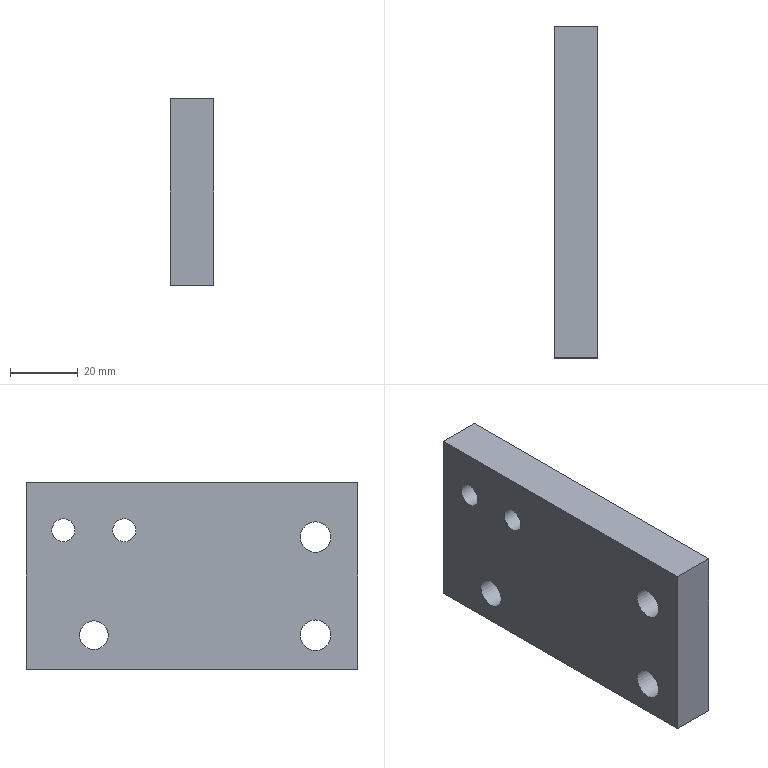Part | NX | features LIN_SOLID_COLOR 2 | 1 solid | 11 faces | box 13 x 98 x 55 mm | volume 66734 mm3 | plane 6 | cylinder 5 | commonest cylinder face diameters 6.8 x2 9 x2 8.5 x1
STEP:
#1=CARTESIAN_POINT('',(938.,-60.,21.25));
#2=VERTEX_POINT('',#1);
#3=CARTESIAN_POINT('',(938.,-60.,17.));
#4=DIRECTION('',(-1.,0.,0.));
#5=DIRECTION('',(0.,0.,1.));
#6=AXIS2_PLACEMENT_3D('',#3,#4,#5);
#7=CIRCLE('',#6,4.25);
#8=EDGE_CURVE('',#2,#2,#7,.T.);
#9=ORIENTED_EDGE('',*,*,#8,.T.);
#10=EDGE_LOOP('',(#9));
#11=FACE_BOUND('',#10,.T.);
#12=CARTESIAN_POINT('',(951.,-60.,12.75));
#13=VERTEX_POINT('',#12);
#14=CARTESIAN_POINT('',(951.,-60.,17.));
#15=DIRECTION('',(1.,0.,0.));
#16=DIRECTION('',(0.,0.,-1.));
#17=AXIS2_PLACEMENT_3D('',#14,#15,#16);
#18=CIRCLE('',#17,4.25);
#19=EDGE_CURVE('',#13,#13,#18,.F.);
#20=ORIENTED_EDGE('',*,*,#19,.F.);
#21=EDGE_LOOP('',(#20));
#22=FACE_BOUND('',#21,.T.);
#23=CARTESIAN_POINT('',(951.,-60.,17.));
#24=DIRECTION('',(-1.,0.,0.));
#25=DIRECTION('',(0.,0.,-1.));
#26=AXIS2_PLACEMENT_3D('',#23,#24,#25);
#27=CYLINDRICAL_SURFACE('',#26,4.25);
#28=ADVANCED_FACE('',(#11,#22),#27,.F.);
#29=CARTESIAN_POINT('',(938.,-69.,51.4));
#30=VERTEX_POINT('',#29);
#31=CARTESIAN_POINT('',(938.,-69.,48.));
#32=DIRECTION('',(-1.,0.,0.));
#33=DIRECTION('',(0.,0.,1.));
#34=AXIS2_PLACEMENT_3D('',#31,#32,#33);
#35=CIRCLE('',#34,3.4);
#36=EDGE_CURVE('',#30,#30,#35,.T.);
#37=ORIENTED_EDGE('',*,*,#36,.T.);
#38=EDGE_LOOP('',(#37));
#39=FACE_BOUND('',#38,.T.);
#40=CARTESIAN_POINT('',(951.,-69.,44.6));
#41=VERTEX_POINT('',#40);
#42=CARTESIAN_POINT('',(951.,-69.,48.));
#43=DIRECTION('',(1.,0.,0.));
#44=DIRECTION('',(0.,0.,-1.));
#45=AXIS2_PLACEMENT_3D('',#42,#43,#44);
#46=CIRCLE('',#45,3.4);
#47=EDGE_CURVE('',#41,#41,#46,.F.);
#48=ORIENTED_EDGE('',*,*,#47,.F.);
#49=EDGE_LOOP('',(#48));
#50=FACE_BOUND('',#49,.T.);
#51=CARTESIAN_POINT('',(951.,-69.,48.));
#52=DIRECTION('',(-1.,0.,0.));
#53=DIRECTION('',(0.,0.,-1.));
#54=AXIS2_PLACEMENT_3D('',#51,#52,#53);
#55=CYLINDRICAL_SURFACE('',#54,3.4);
#56=ADVANCED_FACE('',(#39,#50),#55,.F.);
#57=CARTESIAN_POINT('',(951.,-138.,7.));
#58=VERTEX_POINT('',#57);
#59=CARTESIAN_POINT('',(951.,-138.,62.));
#60=VERTEX_POINT('',#59);
#61=CARTESIAN_POINT('',(951.,-138.,33.449));
#62=DIRECTION('',(0.,0.,-1.));
#63=VECTOR('',#62,1000.);
#64=LINE('',#61,#63);
#65=EDGE_CURVE('',#58,#60,#64,.F.);
#66=ORIENTED_EDGE('',*,*,#65,.T.);
#67=CARTESIAN_POINT('',(938.,-138.,62.));
#68=VERTEX_POINT('',#67);
#69=CARTESIAN_POINT('',(938.5,-138.,62.));
#70=DIRECTION('',(-1.,0.,0.));
#71=VECTOR('',#70,1000.);
#72=LINE('',#69,#71);
#73=EDGE_CURVE('',#60,#68,#72,.T.);
#74=ORIENTED_EDGE('',*,*,#73,.T.);
#75=CARTESIAN_POINT('',(938.,-138.,7.));
#76=VERTEX_POINT('',#75);
#77=CARTESIAN_POINT('',(938.,-138.,33.449));
#78=DIRECTION('',(0.,0.,-1.));
#79=VECTOR('',#78,1000.);
#80=LINE('',#77,#79);
#81=EDGE_CURVE('',#76,#68,#80,.F.);
#82=ORIENTED_EDGE('',*,*,#81,.F.);
#83=CARTESIAN_POINT('',(938.5,-138.,7.));
#84=DIRECTION('',(1.,0.,0.));
#85=VECTOR('',#84,1000.);
#86=LINE('',#83,#85);
#87=EDGE_CURVE('',#76,#58,#86,.T.);
#88=ORIENTED_EDGE('',*,*,#87,.T.);
#89=EDGE_LOOP('',(#66,#74,#82,#88));
#90=FACE_BOUND('',#89,.T.);
#91=CARTESIAN_POINT('',(938.5,-138.,33.449));
#92=DIRECTION('',(0.,-1.,0.));
#93=DIRECTION('',(0.,0.,1.));
#94=AXIS2_PLACEMENT_3D('',#91,#92,#93);
#95=PLANE('',#94);
#96=ADVANCED_FACE('',(#90),#95,.T.);
#97=CARTESIAN_POINT('',(951.,-40.,7.));
#98=VERTEX_POINT('',#97);
#99=CARTESIAN_POINT('',(951.,-175.,7.));
#100=DIRECTION('',(0.,1.,0.));
#101=VECTOR('',#100,1000.);
#102=LINE('',#99,#101);
#103=EDGE_CURVE('',#58,#98,#102,.T.);
#104=ORIENTED_EDGE('',*,*,#103,.F.);
#105=ORIENTED_EDGE('',*,*,#87,.F.);
#106=CARTESIAN_POINT('',(938.,-40.,7.));
#107=VERTEX_POINT('',#106);
#108=CARTESIAN_POINT('',(938.,-175.,7.));
#109=DIRECTION('',(0.,-1.,0.));
#110=VECTOR('',#109,1000.);
#111=LINE('',#108,#110);
#112=EDGE_CURVE('',#107,#76,#111,.T.);
#113=ORIENTED_EDGE('',*,*,#112,.F.);
#114=CARTESIAN_POINT('',(973.,-40.,7.));
#115=DIRECTION('',(-1.,0.,0.));
#116=VECTOR('',#115,1000.);
#117=LINE('',#114,#116);
#118=EDGE_CURVE('',#98,#107,#117,.T.);
#119=ORIENTED_EDGE('',*,*,#118,.F.);
#120=EDGE_LOOP('',(#104,#105,#113,#119));
#121=FACE_BOUND('',#120,.T.);
#122=CARTESIAN_POINT('',(948.5,-25.,7.));
#123=DIRECTION('',(0.,0.,1.));
#124=DIRECTION('',(0.,-1.,0.));
#125=AXIS2_PLACEMENT_3D('',#122,#123,#124);
#126=PLANE('',#125);
#127=ADVANCED_FACE('',(#121),#126,.F.);
#128=CARTESIAN_POINT('',(938.,-40.,62.));
#129=VERTEX_POINT('',#128);
#130=CARTESIAN_POINT('',(938.,-40.,49.449));
#131=DIRECTION('',(0.,0.,-1.));
#132=VECTOR('',#131,1000.);
#133=LINE('',#130,#132);
#134=EDGE_CURVE('',#107,#129,#133,.F.);
#135=ORIENTED_EDGE('',*,*,#134,.T.);
#136=CARTESIAN_POINT('',(951.,-40.,62.));
#137=VERTEX_POINT('',#136);
#138=CARTESIAN_POINT('',(973.,-40.,62.));
#139=DIRECTION('',(1.,0.,0.));
#140=VECTOR('',#139,1000.);
#141=LINE('',#138,#140);
#142=EDGE_CURVE('',#129,#137,#141,.T.);
#143=ORIENTED_EDGE('',*,*,#142,.T.);
#144=CARTESIAN_POINT('',(951.,-40.,33.449));
#145=DIRECTION('',(0.,0.,-1.));
#146=VECTOR('',#145,1000.);
#147=LINE('',#144,#146);
#148=EDGE_CURVE('',#98,#137,#147,.F.);
#149=ORIENTED_EDGE('',*,*,#148,.F.);
#150=ORIENTED_EDGE('',*,*,#118,.T.);
#151=EDGE_LOOP('',(#135,#143,#149,#150));
#152=FACE_BOUND('',#151,.T.);
#153=CARTESIAN_POINT('',(973.,-40.,49.449));
#154=DIRECTION('',(0.,1.,0.));
#155=DIRECTION('',(1.,0.,0.));
#156=AXIS2_PLACEMENT_3D('',#153,#154,#155);
#157=PLANE('',#156);
#158=ADVANCED_FACE('',(#152),#157,.T.);
#159=CARTESIAN_POINT('',(938.,-175.,62.));
#160=DIRECTION('',(0.,1.,0.));
#161=VECTOR('',#160,1000.);
#162=LINE('',#159,#161);
#163=EDGE_CURVE('',#68,#129,#162,.T.);
#164=ORIENTED_EDGE('',*,*,#163,.F.);
#165=ORIENTED_EDGE('',*,*,#73,.F.);
#166=CARTESIAN_POINT('',(951.,-175.,62.));
#167=DIRECTION('',(0.,-1.,0.));
#168=VECTOR('',#167,1000.);
#169=LINE('',#166,#168);
#170=EDGE_CURVE('',#137,#60,#169,.T.);
#171=ORIENTED_EDGE('',*,*,#170,.F.);
#172=ORIENTED_EDGE('',*,*,#142,.F.);
#173=EDGE_LOOP('',(#164,#165,#171,#172));
#174=FACE_BOUND('',#173,.T.);
#175=CARTESIAN_POINT('',(938.5,-127.,62.));
#176=DIRECTION('',(0.,0.,-1.));
#177=DIRECTION('',(0.,1.,0.));
#178=AXIS2_PLACEMENT_3D('',#175,#176,#177);
#179=PLANE('',#178);
#180=ADVANCED_FACE('',(#174),#179,.F.);
#181=CARTESIAN_POINT('',(938.,-51.,51.4));
#182=VERTEX_POINT('',#181);
#183=CARTESIAN_POINT('',(938.,-51.,48.));
#184=DIRECTION('',(-1.,0.,0.));
#185=DIRECTION('',(0.,0.,1.));
#186=AXIS2_PLACEMENT_3D('',#183,#184,#185);
#187=CIRCLE('',#186,3.4);
#188=EDGE_CURVE('',#182,#182,#187,.T.);
#189=ORIENTED_EDGE('',*,*,#188,.T.);
#190=EDGE_LOOP('',(#189));
#191=FACE_BOUND('',#190,.T.);
#192=CARTESIAN_POINT('',(951.,-51.,44.6));
#193=VERTEX_POINT('',#192);
#194=CARTESIAN_POINT('',(951.,-51.,48.));
#195=DIRECTION('',(1.,0.,0.));
#196=DIRECTION('',(0.,0.,-1.));
#197=AXIS2_PLACEMENT_3D('',#194,#195,#196);
#198=CIRCLE('',#197,3.4);
#199=EDGE_CURVE('',#193,#193,#198,.F.);
#200=ORIENTED_EDGE('',*,*,#199,.F.);
#201=EDGE_LOOP('',(#200));
#202=FACE_BOUND('',#201,.T.);
#203=CARTESIAN_POINT('',(951.,-51.,48.));
#204=DIRECTION('',(-1.,0.,0.));
#205=DIRECTION('',(0.,0.,-1.));
#206=AXIS2_PLACEMENT_3D('',#203,#204,#205);
#207=CYLINDRICAL_SURFACE('',#206,3.4);
#208=ADVANCED_FACE('',(#191,#202),#207,.F.);
#209=CARTESIAN_POINT('',(951.,-125.5,12.5));
#210=VERTEX_POINT('',#209);
#211=CARTESIAN_POINT('',(951.,-125.5,17.));
#212=DIRECTION('',(1.,0.,0.));
#213=DIRECTION('',(0.,0.,-1.));
#214=AXIS2_PLACEMENT_3D('',#211,#212,#213);
#215=CIRCLE('',#214,4.5);
#216=EDGE_CURVE('',#210,#210,#215,.T.);
#217=ORIENTED_EDGE('',*,*,#216,.T.);
#218=EDGE_LOOP('',(#217));
#219=FACE_BOUND('',#218,.T.);
#220=CARTESIAN_POINT('',(938.,-125.5,21.5));
#221=VERTEX_POINT('',#220);
#222=CARTESIAN_POINT('',(938.,-125.5,17.));
#223=DIRECTION('',(-1.,0.,0.));
#224=DIRECTION('',(0.,0.,1.));
#225=AXIS2_PLACEMENT_3D('',#222,#223,#224);
#226=CIRCLE('',#225,4.5);
#227=EDGE_CURVE('',#221,#221,#226,.F.);
#228=ORIENTED_EDGE('',*,*,#227,.F.);
#229=EDGE_LOOP('',(#228));
#230=FACE_BOUND('',#229,.T.);
#231=CARTESIAN_POINT('',(938.,-125.5,17.));
#232=DIRECTION('',(1.,0.,0.));
#233=DIRECTION('',(0.,0.,1.));
#234=AXIS2_PLACEMENT_3D('',#231,#232,#233);
#235=CYLINDRICAL_SURFACE('',#234,4.5);
#236=ADVANCED_FACE('',(#219,#230),#235,.F.);
#237=CARTESIAN_POINT('',(951.,-125.5,41.5));
#238=VERTEX_POINT('',#237);
#239=CARTESIAN_POINT('',(951.,-125.5,46.));
#240=DIRECTION('',(1.,0.,0.));
#241=DIRECTION('',(0.,0.,-1.));
#242=AXIS2_PLACEMENT_3D('',#239,#240,#241);
#243=CIRCLE('',#242,4.5);
#244=EDGE_CURVE('',#238,#238,#243,.T.);
#245=ORIENTED_EDGE('',*,*,#244,.F.);
#246=EDGE_LOOP('',(#245));
#247=FACE_BOUND('',#246,.T.);
#248=ORIENTED_EDGE('',*,*,#216,.F.);
#249=EDGE_LOOP('',(#248));
#250=FACE_BOUND('',#249,.T.);
#251=ORIENTED_EDGE('',*,*,#199,.T.);
#252=EDGE_LOOP('',(#251));
#253=FACE_BOUND('',#252,.T.);
#254=ORIENTED_EDGE('',*,*,#170,.T.);
#255=ORIENTED_EDGE('',*,*,#65,.F.);
#256=ORIENTED_EDGE('',*,*,#103,.T.);
#257=ORIENTED_EDGE('',*,*,#148,.T.);
#258=EDGE_LOOP('',(#254,#255,#256,#257));
#259=FACE_BOUND('',#258,.T.);
#260=ORIENTED_EDGE('',*,*,#47,.T.);
#261=EDGE_LOOP('',(#260));
#262=FACE_BOUND('',#261,.T.);
#263=ORIENTED_EDGE('',*,*,#19,.T.);
#264=EDGE_LOOP('',(#263));
#265=FACE_BOUND('',#264,.T.);
#266=CARTESIAN_POINT('',(951.,-175.,33.449));
#267=DIRECTION('',(1.,0.,0.));
#268=DIRECTION('',(0.,0.,1.));
#269=AXIS2_PLACEMENT_3D('',#266,#267,#268);
#270=PLANE('',#269);
#271=ADVANCED_FACE('',(#247,#250,#253,#259,#262,#265),#270,.T.);
#272=CARTESIAN_POINT('',(938.,-125.5,50.5));
#273=VERTEX_POINT('',#272);
#274=CARTESIAN_POINT('',(938.,-125.5,46.));
#275=DIRECTION('',(-1.,0.,0.));
#276=DIRECTION('',(0.,0.,1.));
#277=AXIS2_PLACEMENT_3D('',#274,#275,#276);
#278=CIRCLE('',#277,4.5);
#279=EDGE_CURVE('',#273,#273,#278,.T.);
#280=ORIENTED_EDGE('',*,*,#279,.F.);
#281=EDGE_LOOP('',(#280));
#282=FACE_BOUND('',#281,.T.);
#283=ORIENTED_EDGE('',*,*,#112,.T.);
#284=ORIENTED_EDGE('',*,*,#81,.T.);
#285=ORIENTED_EDGE('',*,*,#163,.T.);
#286=ORIENTED_EDGE('',*,*,#134,.F.);
#287=EDGE_LOOP('',(#283,#284,#285,#286));
#288=FACE_BOUND('',#287,.T.);
#289=ORIENTED_EDGE('',*,*,#36,.F.);
#290=EDGE_LOOP('',(#289));
#291=FACE_BOUND('',#290,.T.);
#292=ORIENTED_EDGE('',*,*,#188,.F.);
#293=EDGE_LOOP('',(#292));
#294=FACE_BOUND('',#293,.T.);
#295=ORIENTED_EDGE('',*,*,#8,.F.);
#296=EDGE_LOOP('',(#295));
#297=FACE_BOUND('',#296,.T.);
#298=ORIENTED_EDGE('',*,*,#227,.T.);
#299=EDGE_LOOP('',(#298));
#300=FACE_BOUND('',#299,.T.);
#301=CARTESIAN_POINT('',(938.,-175.,33.449));
#302=DIRECTION('',(-1.,0.,0.));
#303=DIRECTION('',(0.,0.,-1.));
#304=AXIS2_PLACEMENT_3D('',#301,#302,#303);
#305=PLANE('',#304);
#306=ADVANCED_FACE('',(#282,#288,#291,#294,#297,#300),#305,.T.);
#307=ORIENTED_EDGE('',*,*,#244,.T.);
#308=EDGE_LOOP('',(#307));
#309=FACE_BOUND('',#308,.T.);
#310=ORIENTED_EDGE('',*,*,#279,.T.);
#311=EDGE_LOOP('',(#310));
#312=FACE_BOUND('',#311,.T.);
#313=CARTESIAN_POINT('',(938.,-125.5,46.));
#314=DIRECTION('',(1.,0.,0.));
#315=DIRECTION('',(0.,0.,1.));
#316=AXIS2_PLACEMENT_3D('',#313,#314,#315);
#317=CYLINDRICAL_SURFACE('',#316,4.5);
#318=ADVANCED_FACE('',(#309,#312),#317,.F.);
#319=CLOSED_SHELL('',(#28,#56,#96,#127,#158,#180,#208,#236,#271,#306,#318));
#320=MANIFOLD_SOLID_BREP('',#319);
#321=(LENGTH_UNIT()NAMED_UNIT(*)SI_UNIT(.MILLI.,.METRE.));
#322=UNCERTAINTY_MEASURE_WITH_UNIT(LENGTH_MEASURE(0.00001),#321,'','');
#323=(NAMED_UNIT(*)PLANE_ANGLE_UNIT()SI_UNIT($,.RADIAN.));
#324=(NAMED_UNIT(*)SI_UNIT($,.STERADIAN.)SOLID_ANGLE_UNIT());
#325=(GEOMETRIC_REPRESENTATION_CONTEXT(3)GLOBAL_UNCERTAINTY_ASSIGNED_CONTEXT((#322))GLOBAL_UNIT_ASSIGNED_CONTEXT((#321,#323,#324))REPRESENTATION_CONTEXT('',''));
#326=ADVANCED_BREP_SHAPE_REPRESENTATION('',(#320),#325);